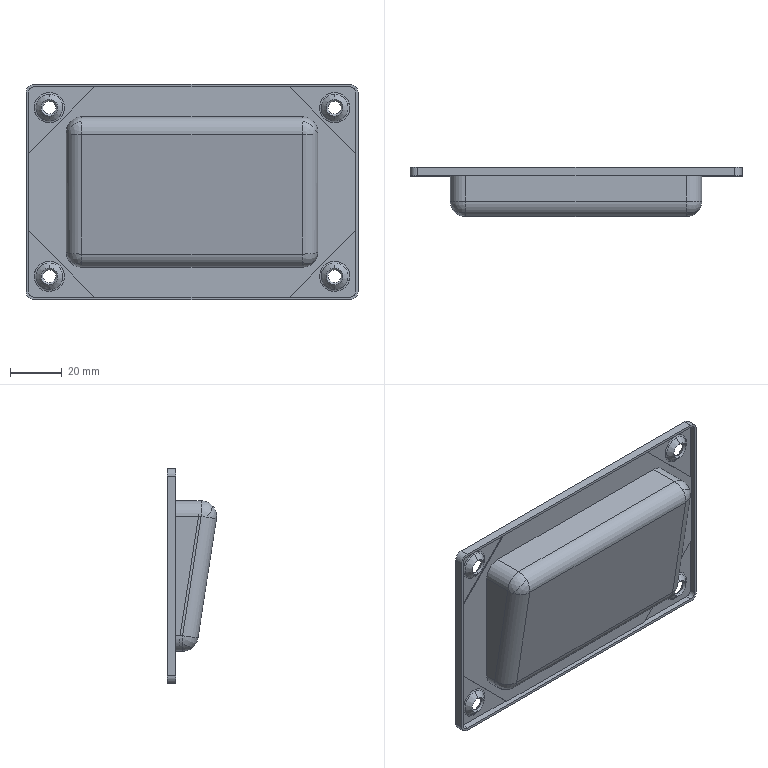Part | STEP file | door handle XAC81_A128 | 1 solid | 130 faces | box 128 x 19.001 x 83 mm | volume 21652 mm3 | plane 44 | cylinder 30 | cone 24 | sphere 16 | torus 16 | commonest cylinder face diameters 6 x8 11 x8 12 x8 4 x4 2.4 x2